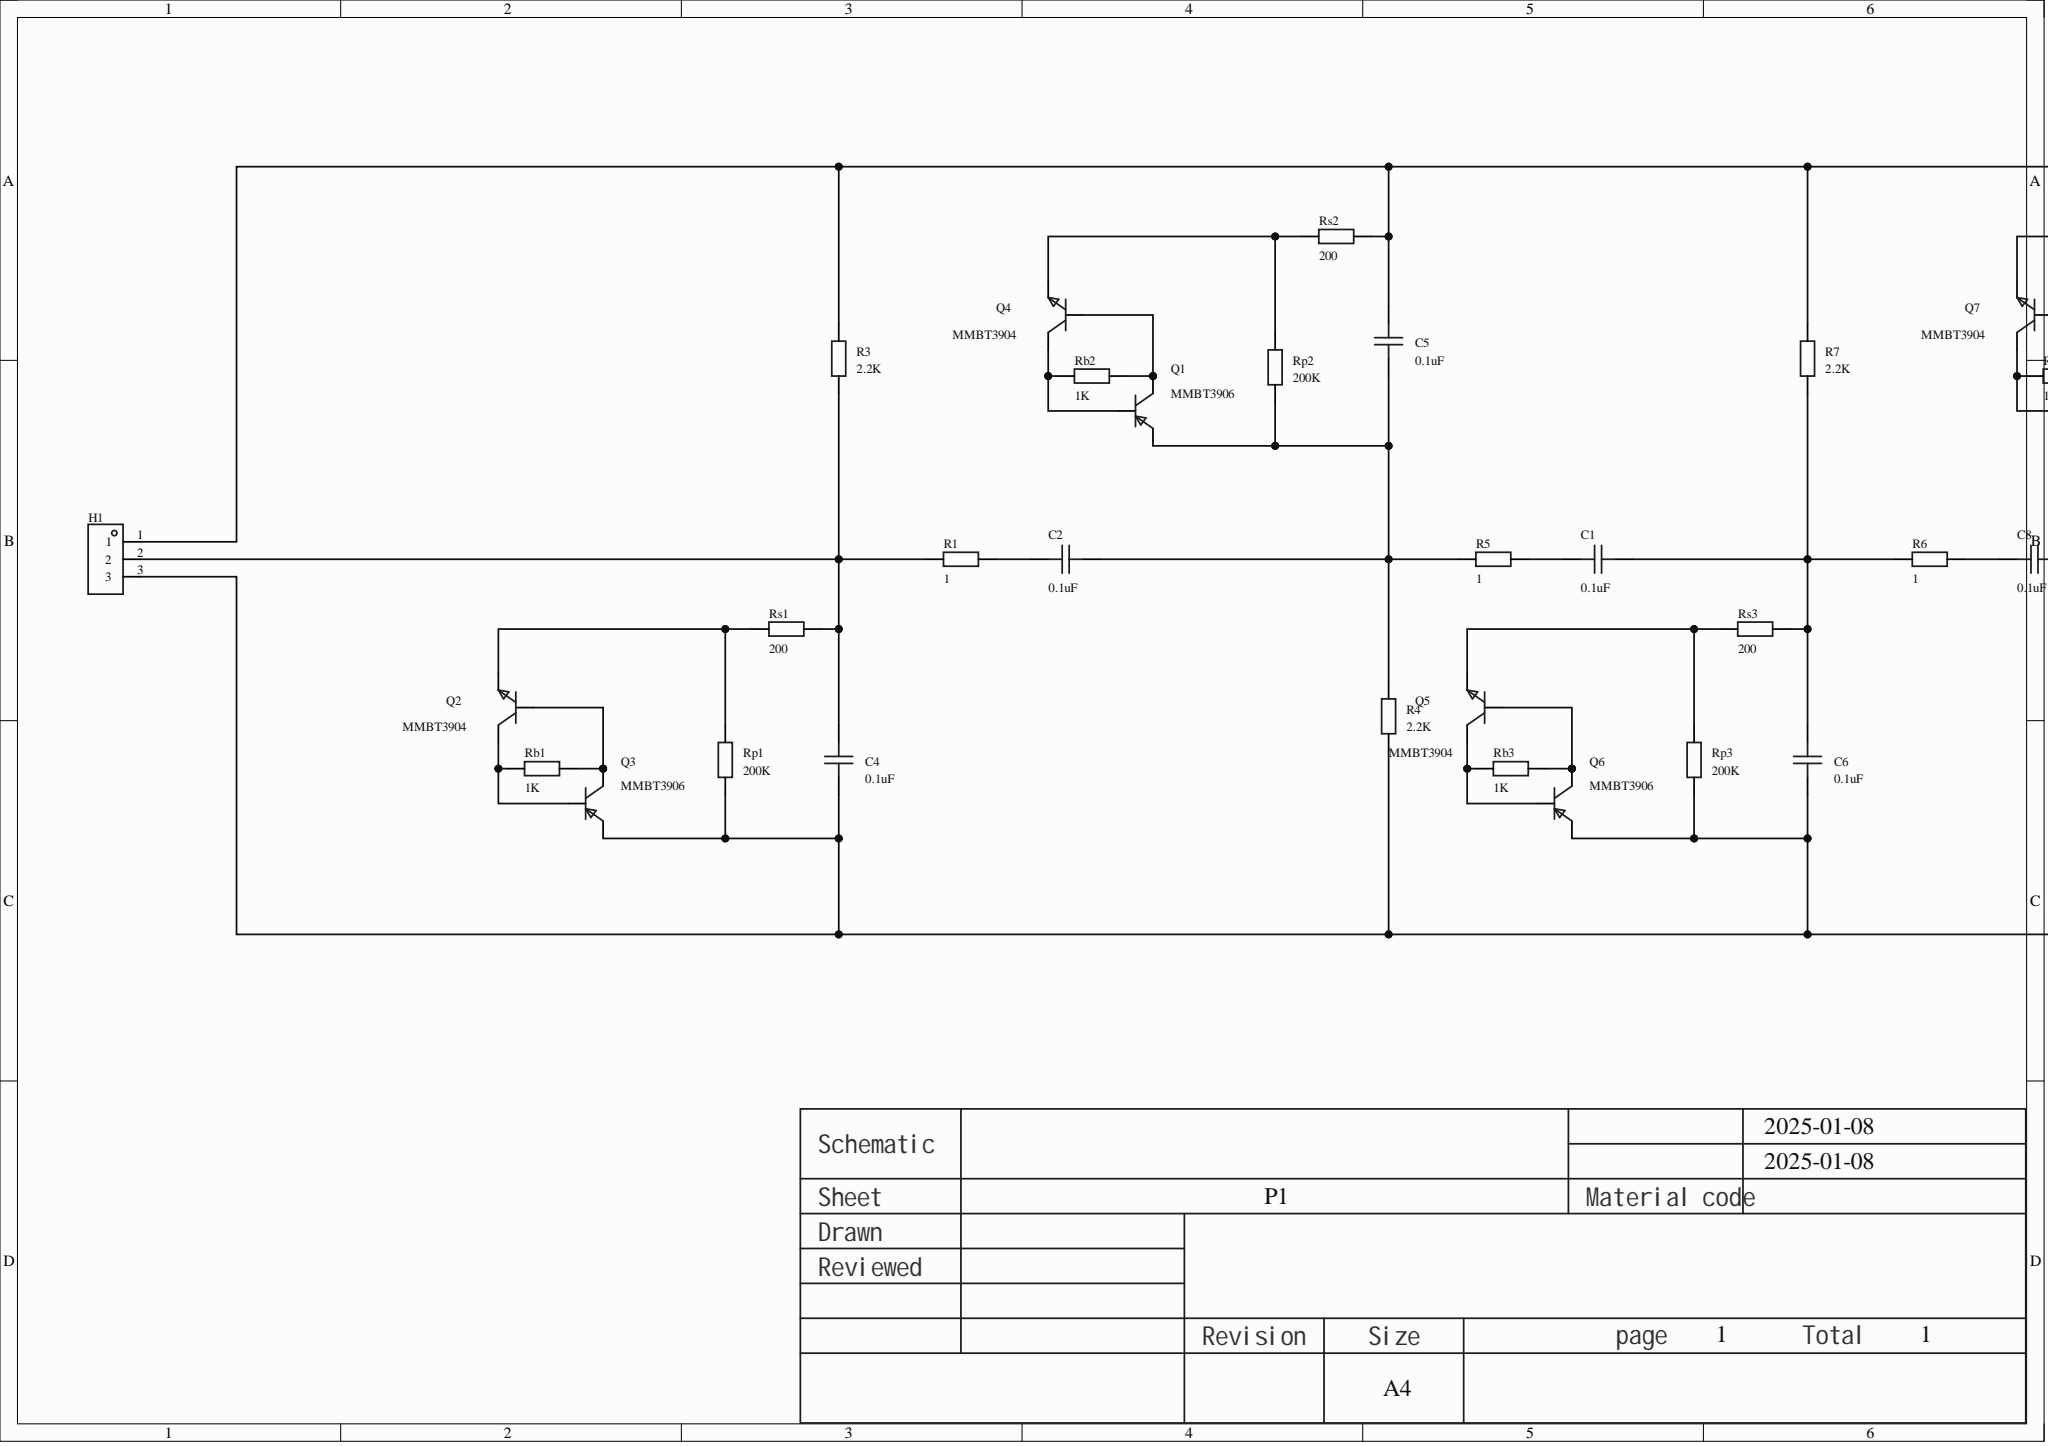Circuit board | Altium Designer | 257 parts | 141 nets
Bill of materials:
Comment,Description,Designator,Footprint,LibRef,Quantity
"0.1uF","","C1, C2, C4, C5, C6, C7, C8, C9, C10, C11, C12, C13, C14, C15, C16, C17, C18, C19, C20, C21, C22, C23, C24, C25, C26, C27, C28, C29, C30, C31, C32, C33, C34, C35, C36, C37, C38, C39, C40, C41, C42, C43, C44, C45, C46, C47, C48, C49, C50, C51, C52, C53, C54, C55, C56","C0402","CAP_0402","55"
"","","H1","HDR-TH_3P-P2.54-V-M","HDR-M_2.54_1x3P","1"
"","","H2, H3, H4, H5, H6, H7","HDR-TH_2P-P2.54-V-M-1","HDR-M_2.54_1x2P","6"
"MMBT3906","Transistor type:-;Collector current(Ic):-;Collector-emitter breakdown voltage(Vceo):-;Power(Pd):-;","Q1, Q3, Q6, Q8, Q10, Q12, Q14, Q16, Q18, Q20, Q22, Q24, Q26, Q28, Q30, Q32, Q34, Q36, Q38, Q40, Q42, Q44, Q46, Q48, Q50, Q52, Q54, Q56","SOT-23-3_L2.9-W1.3-P1.90-LS2.4-BR","MMBT3906-13-01-F","28"
"MMBT3904","晶体管类型:NPN;集电极电流(Ic):200mA;集射极击穿电压(Vceo):40V;功率(Pd):200mW;直流电流增益(hFE@Ic,Vce):100@10mA,1V;","Q2, Q4, Q5, Q7, Q9, Q11, Q13, Q15, Q17, Q19, Q21, Q23, Q25, Q27, Q29, Q31, Q33, Q35, Q37, Q39, Q41, Q43, Q45, Q47, Q49, Q51, Q53, Q55","SOT-23-3_L2.9-W1.3-P1.90-LS2.4-BR","MMBT3904(RANGE:100-300)","28"
"1","","R1, R5, R6, R8, R10, R12, R14, R16, R18, R20, R22, R24, R26, R28, R30, R32, R34, R36, R38, R40, R42, R44, R46, R48, R50, R52, R54","R0402","Res_0402","27"
"2.2K","","R3, R4, R7, R9, R11, R13, R15, R17, R19, R21, R23, R25, R27, R29, R31, R33, R35, R37, R39, R41, R43, R45, R47, R49, R51, R53, R55, R56","R0402","Res_0402","28"
"1K","","Rb1, Rb2, Rb3, Rb4, Rb5, Rb6, Rb7, Rb8, Rb9, Rb10, Rb11, Rb12, Rb13, Rb14, Rb15, Rb16, Rb17, Rb18, Rb19, Rb20, Rb21, Rb22, Rb23, Rb24, Rb25, Rb26, Rb27, Rb28","R0402","Res_0402","28"
"200K","","Rp1, Rp2, Rp3, Rp4, Rp5, Rp6, Rp7, Rp8, Rp9, Rp10, Rp11, Rp12, Rp13, Rp14, Rp15, Rp16, Rp17, Rp18, Rp19, Rp20, Rp21, Rp22, Rp23, Rp24, Rp25, Rp26, Rp27, Rp28","R0402","Res_0402","28"
"200","","Rs1, Rs2, Rs3, Rs4, Rs5, Rs6, Rs7, Rs8, Rs9, Rs10, Rs11, Rs12, Rs13, Rs14, Rs15, Rs16, Rs17, Rs18, Rs19, Rs20, Rs21, Rs22, Rs23, Rs24, Rs25, Rs26, Rs27, Rs28","R0402","Res_0402","28"
Netlist (Protel format):
[
C1
C0402
0.1uF



]
[
C2
C0402
0.1uF



]
[
C4
C0402
0.1uF



]
[
C5
C0402
0.1uF



]
[
C6
C0402
0.1uF



]
[
C7
C0402
0.1uF



]
[
C8
C0402
0.1uF



]
[
C9
C0402
0.1uF



]
[
C10
C0402
0.1uF



]
[
C11
C0402
0.1uF



]
[
C12
C0402
0.1uF



]
[
C13
C0402
0.1uF



]
[
C14
C0402
0.1uF



]
[
C15
C0402
0.1uF



]
[
C16
C0402
0.1uF



]
[
C17
C0402
0.1uF



]
[
C18
C0402
0.1uF



]
[
C19
C0402
0.1uF



]
[
C20
C0402
0.1uF



]
[
C21
C0402
0.1uF



]
[
C22
C0402
0.1uF



]
[
C23
C0402
0.1uF



]
[
C24
C0402
0.1uF



]
[
C25
C0402
0.1uF



]
[
C26
C0402
0.1uF



]
[
C27
C0402
0.1uF



]
[
C28
C0402
0.1uF



]
[
C29
C0402
0.1uF



]
[
C30
C0402
0.1uF



]
[
C31
C0402
0.1uF



]
[
C32
C0402
0.1uF



]
[
C33
C0402
0.1uF



]
[
C34
C0402
0.1uF



]
[
C35
C0402
0.1uF



]
[
C36
C0402
0.1uF



]
[
C37
C0402
0.1uF



]
[
C38
C0402
0.1uF



]
[
C39
C0402
0.1uF



]
[
C40
C0402
0.1uF



]
[
C41
C0402
0.1uF



]
[
C42
C0402
0.1uF



]
[
C43
C0402
0.1uF



]
[
C44
C0402
0.1uF



]
[
C45
C0402
0.1uF



]
[
C46
C0402
0.1uF



]
[
C47
C0402
0.1uF



]
[
C48
C0402
0.1uF



]
[
C49
C0402
0.1uF



]
[
C50
C0402
0.1uF



]
[
C51
C0402
0.1uF



]
[
C52
C0402
0.1uF



]
[
C53
C0402
0.1uF



]
[
C54
C0402
0.1uF



]
[
C55
C0402
0.1uF



]
[
C56
C0402
0.1uF



]
[
H1
HDR-TH_3P-P2.54-V-M




]
[
H2
HDR-TH_2P-P2.54-V-M-1




]
[
H3
HDR-TH_2P-P2.54-V-M-1




]
[
H4
HDR-TH_2P-P2.54-V-M-1




]
[
H5
HDR-TH_2P-P2.54-V-M-1




]
[
H6
HDR-TH_2P-P2.54-V-M-1




]
[
H7
HDR-TH_2P-P2.54-V-M-1




]
[
Q1
SOT-23-3_L2.9-W1.3-P1.90-LS2.4-BR
MMBT3906



]
[
Q2
SOT-23-3_L2.9-W1.3-P1.90-LS2.4-BR
MMBT3904



]
[
Q3
SOT-23-3_L2.9-W1.3-P1.90-LS2.4-BR
MMBT3906



]
[
Q4
SOT-23-3_L2.9-W1.3-P1.90-LS2.4-BR
MMBT3904



]
[
Q5
SOT-23-3_L2.9-W1.3-P1.90-LS2.4-BR
MMBT3904



]
[
Q6
SOT-23-3_L2.9-W1.3-P1.90-LS2.4-BR
MMBT3906



]
[
Q7
SOT-23-3_L2.9-W1.3-P1.90-LS2.4-BR
MMBT3904



]
[
Q8
SOT-23-3_L2.9-W1.3-P1.90-LS2.4-BR
MMBT3906



]
[
Q9
SOT-23-3_L2.9-W1.3-P1.90-LS2.4-BR
MMBT3904



]
[
Q10
SOT-23-3_L2.9-W1.3-P1.90-LS2.4-BR
MMBT3906



]
[
Q11
SOT-23-3_L2.9-W1.3-P1.90-LS2.4-BR
MMBT3904



]
[
Q12
SOT-23-3_L2.9-W1.3-P1.90-LS2.4-BR
MMBT3906



]
[
Q13
SOT-23-3_L2.9-W1.3-P1.90-LS2.4-BR
MMBT3904



]
[
Q14
SOT-23-3_L2.9-W1.3-P1.90-LS2.4-BR
MMBT3906



]
[
Q15
SOT-23-3_L2.9-W1.3-P1.90-LS2.4-BR
MMBT3904



]
[
Q16
SOT-23-3_L2.9-W1.3-P1.90-LS2.4-BR
MMBT3906



]
[
Q17
SOT-23-3_L2.9-W1.3-P1.90-LS2.4-BR
MMBT3904



]
[
Q18
SOT-23-3_L2.9-W1.3-P1.90-LS2.4-BR
MMBT3906



]
[
Q19
SOT-23-3_L2.9-W1.3-P1.90-LS2.4-BR
MMBT3904



]
[
Q20
SOT-23-3_L2.9-W1.3-P1.90-LS2.4-BR
MMBT3906



]
[
Q21
SOT-23-3_L2.9-W1.3-P1.90-LS2.4-BR
MMBT3904



]
[
Q22
SOT-23-3_L2.9-W1.3-P1.90-LS2.4-BR
MMBT3906



]
[
Q23
SOT-23-3_L2.9-W1.3-P1.90-LS2.4-BR
MMBT3904



]
[
Q24
SOT-23-3_L2.9-W1.3-P1.90-LS2.4-BR
MMBT3906



]
[
Q25
SOT-23-3_L2.9-W1.3-P1.90-LS2.4-BR
MMBT3904



]
[
Q26
SOT-23-3_L2.9-W1.3-P1.90-LS2.4-BR
MMBT3906



]
[
Q27
SOT-23-3_L2.9-W1.3-P1.90-LS2.4-BR
MMBT3904



]
[
Q28
SOT-23-3_L2.9-W1.3-P1.90-LS2.4-BR
MMBT3906



]
[
Q29
SOT-23-3_L2.9-W1.3-P1.90-LS2.4-BR
MMBT3904



]
[
Q30
SOT-23-3_L2.9-W1.3-P1.90-LS2.4-BR
MMBT3906



]
[
Q31
SOT-23-3_L2.9-W1.3-P1.90-LS2.4-BR
MMBT3904



]
[
Q32
SOT-23-3_L2.9-W1.3-P1.90-LS2.4-BR
MMBT3906



]
[
Q33
SOT-23-3_L2.9-W1.3-P1.90-LS2.4-BR
MMBT3904



]
[
Q34
SOT-23-3_L2.9-W1.3-P1.90-LS2.4-BR
MMBT3906



]
[
Q35
SOT-23-3_L2.9-W1.3-P1.90-LS2.4-BR
MMBT3904



]
[
Q36
SOT-23-3_L2.9-W1.3-P1.90-LS2.4-BR
MMBT3906



]
[
Q37
SOT-23-3_L2.9-W1.3-P1.90-LS2.4-BR
MMBT3904



]
[
Q38
SOT-23-3_L2.9-W1.3-P1.90-LS2.4-BR
MMBT3906



]
[
Q39
SOT-23-3_L2.9-W1.3-P1.90-LS2.4-BR
MMBT3904



]
[
Q40
SOT-23-3_L2.9-W1.3-P1.90-LS2.4-BR
MMBT3906



]
[
Q41
SOT-23-3_L2.9-W1.3-P1.90-LS2.4-BR
MMBT3904



]
[
Q42
SOT-23-3_L2.9-W1.3-P1.90-LS2.4-BR
MMBT3906



]
[
Q43
SOT-23-3_L2.9-W1.3-P1.90-LS2.4-BR
MMBT3904



]
[
Q44
SOT-23-3_L2.9-W1.3-P1.90-LS2.4-BR
MMBT3906



]
[
Q45
SOT-23-3_L2.9-W1.3-P1.90-LS2.4-BR
MMBT3904



]
[
Q46
SOT-23-3_L2.9-W1.3-P1.90-LS2.4-BR
MMBT3906



]
[
Q47
SOT-23-3_L2.9-W1.3-P1.90-LS2.4-BR
MMBT3904



]
[
Q48
SOT-23-3_L2.9-W1.3-P1.90-LS2.4-BR
MMBT3906



]
[
Q49
SOT-23-3_L2.9-W1.3-P1.90-LS2.4-BR
MMBT3904



]
[
Q50
SOT-23-3_L2.9-W1.3-P1.90-LS2.4-BR
MMBT3906



]
[
Q51
SOT-23-3_L2.9-W1.3-P1.90-LS2.4-BR
MMBT3904



]
[
Q52
SOT-23-3_L2.9-W1.3-P1.90-LS2.4-BR
MMBT3906



]
[
Q53
SOT-23-3_L2.9-W1.3-P1.90-LS2.4-BR
MMBT3904



]
[
Q54
SOT-23-3_L2.9-W1.3-P1.90-LS2.4-BR
MMBT3906



]
[
Q55
SOT-23-3_L2.9-W1.3-P1.90-LS2.4-BR
MMBT3904



]
[
Q56
SOT-23-3_L2.9-W1.3-P1.90-LS2.4-BR
MMBT3906



]
[
R1
R0402
1



]
[
R3
R0402
2.2K



]
[
R4
R0402
2.2K



]
[
R5
R0402
1



]
[
R6
R0402
1



]
[
R7
R0402
2.2K



]
[
R8
R0402
1



]
[
R9
R0402
2.2K



]
[
R10
R0402
1



]
[
R11
R0402
2.2K



]
[
R12
R0402
1



]
[
R13
R0402
2.2K



]
[
R14
R0402
1



]
[
R15
R0402
2.2K



]
[
R16
R0402
1



]
[
R17
R0402
2.2K



]
[
R18
R0402
1



]
[
R19
R0402
2.2K



]
[
R20
R0402
1



]
[
R21
R0402
2.2K



]
[
R22
R0402
1



]
[
R23
R0402
2.2K



]
[
R24
R0402
1



]
[
R25
R0402
2.2K



]
[
R26
R0402
1



]
[
R27
R0402
2.2K



]
[
R28
R0402
1



]
[
R29
R0402
2.2K



]
[
R30
R0402
1



]
[
R31
R0402
2.2K



]
[
R32
R0402
1



]
[
R33
R0402
2.2K



]
[
R34
R0402
1



]
[
R35
R0402
2.2K



]
[
R36
R0402
1



]
[
R37
R0402
2.2K



]
[
R38
R0402
1



]
[
R39
R0402
2.2K



]
[
R40
R0402
1



]
[
R41
R0402
2.2K



]
[
R42
R0402
1



]
[
R43
R0402
2.2K



]
[
R44
R0402
1



]
[
R45
R0402
2.2K



]
[
R46
R0402
1



]
[
R47
R0402
2.2K



]
[
R48
R0402
1



]
[
R49
R0402
2.2K



]
[
R50
R0402
1



]
[
R51
R0402
2.2K



]
[
R52
R0402
1



]
[
R53
R0402
2.2K



]
[
R54
R0402
1



]
[
R55
R0402
2.2K



]
[
R56
R0402
2.2K



]
[
Rb1
R0402
1K



]
[
Rb2
R0402
1K



]
[
Rb3
R0402
1K



]
[
Rb4
R0402
1K



]
[
Rb5
R0402
1K



]
[
Rb6
R0402
1K



]
[
Rb7
R0402
1K



]
[
Rb8
R0402
1K



]
[
Rb9
R0402
1K



]
[
Rb10
R0402
1K



]
[
Rb11
R0402
1K



]
[
Rb12
R0402
1K



]
[
Rb13
R0402
1K



]
[
Rb14
R0402
1K



]
[
Rb15
R0402
1K



]
[
Rb16
R0402
1K



]
[
Rb17
R0402
1K



]
[
Rb18
R0402
1K



]
[
Rb19
R0402
1K



]
[
Rb20
R0402
1K



]
[
Rb21
R0402
1K



]
[
Rb22
R0402
1K



]
[
Rb23
R0402
1K



]
[
Rb24
R0402
1K



]
[
Rb25
R0402
1K



]
[
Rb26
R0402
1K



]
[
Rb27
R0402
1K



]
[
Rb28
R0402
1K



]
[
Rp1
R0402
200K



]
[
Rp2
R0402
200K



]
[
Rp3
R0402
200K



]
[
Rp4
R0402
200K



]
[
Rp5
R0402
200K



]
[
Rp6
R0402
200K



]
[
Rp7
R0402
200K



]
[
Rp8
R0402
200K



]
[
Rp9
R0402
200K



]
[
Rp10
R0402
200K



]
[
Rp11
R0402
200K



]
[
Rp12
R0402
200K



]
[
Rp13
R0402
200K



]
[
Rp14
R0402
200K



]
[
Rp15
R0402
200K



]
[
Rp16
R0402
200K



]
[
Rp17
R0402
200K



]
[
Rp18
R0402
200K



]
[
Rp19
R0402
200K



]
[
Rp20
R0402
200K



]
[
Rp21
R0402
200K



]
[
Rp22
R0402
200K



]
[
Rp23
R0402
200K



]
[
Rp24
R0402
200K



]
[
Rp25
R0402
200K



]
[
Rp26
R0402
200K



]
[
Rp27
R0402
200K



]
[
Rp28
R0402
200K



]
[
Rs1
R0402
200



]
[
Rs2
R0402
200



]
[
Rs3
R0402
200



]
[
Rs4
R0402
200



]
[
Rs5
R0402
200



]
[
Rs6
R0402
200



]
[
Rs7
R0402
200



]
[
Rs8
R0402
200



]
[
Rs9
R0402
200



]
[
Rs10
R0402
200



]
[
Rs11
R0402
200



]
[
Rs12
R0402
200



]
[
Rs13
R0402
200



]
[
Rs14
R0402
200



]
[
Rs15
R0402
200



]
[
Rs16
R0402
200



]
[
Rs17
R0402
200



]
[
Rs18
R0402
200



]
[
Rs19
R0402
200



]
[
Rs20
R0402
200



]
[
Rs21
R0402
200



]
[
Rs22
R0402
200



]
[
Rs23
R0402
200



]
[
Rs24
R0402
200



]
[
Rs25
R0402
200



]
[
Rs26
R0402
200



]
[
Rs27
R0402
200



]
[
Rs28
R0402
200



]
(
NetQ55_3
Q55-3
Q56-1
Rb28-2
)
(
NetQ55_2
Q55-2
Rp28-2
Rs28-1
)
(
NetQ55_1
Q55-1
Q56-3
Rb28-1
)
(
NetQ53_3
Q53-3
Q54-1
Rb27-2
)
(
NetQ53_2
Q53-2
Rp27-2
Rs27-1
)
(
NetQ53_1
Q53-1
Q54-3
Rb27-1
)
(
NetQ51_3
Q51-3
Q52-1
Rb26-2
)
(
NetQ51_2
Q51-2
Rp26-2
Rs26-1
)
(
NetQ51_1
Q51-1
Q52-3
Rb26-1
)
(
NetQ49_3
Q49-3
Q50-1
Rb25-2
)
(
NetQ49_2
Q49-2
Rp25-2
Rs25-1
)
(
NetQ49_1
Q49-1
Q50-3
Rb25-1
)
(
NetQ47_3
Q47-3
Q48-1
Rb24-2
)
(
NetQ47_1
Q47-1
Q48-3
Rb24-1
)
(
NetQ45_3
Q45-3
Q46-1
Rb23-2
)
(
NetQ45_2
Q45-2
Rp23-2
Rs23-1
)
(
NetQ45_1
Q45-1
Q46-3
Rb23-1
)
(
NetQ43_3
Q43-3
Q44-1
Rb22-2
)
(
NetQ43_2
Q43-2
Rp22-2
Rs22-1
)
(
NetQ43_1
Q43-1
Q44-3
Rb22-1
)
(
NetQ41_3
Q41-3
Q42-1
Rb21-2
)
(
NetQ41_2
Q41-2
Rp21-2
Rs21-1
)
(
NetQ41_1
Q41-1
Q42-3
Rb21-1
)
(
NetQ39_3
Q39-3
Q40-1
Rb20-2
)
(
NetQ39_1
Q39-1
Q40-3
Rb20-1
)
(
NetQ37_3
Q37-3
Q38-1
Rb19-2
)
(
NetQ37_2
Q37-2
Rp19-2
Rs19-1
)
(
NetQ37_1
Q37-1
Q38-3
Rb19-1
)
(
NetQ35_3
Q35-3
Q36-1
Rb18-2
)
(
NetQ35_2
Q35-2
Rp18-2
Rs18-1
)
(
NetQ35_1
Q35-1
Q36-3
Rb18-1
)
(
NetQ33_3
Q33-3
Q34-1
Rb17-2
)
(
NetQ33_2
Q33-2
Rp17-2
Rs17-1
)
(
NetQ33_1
Q33-1
Q34-3
Rb17-1
)
(
NetQ31_3
Q31-3
Q32-1
Rb16-2
)
(
NetQ31_1
Q31-1
Q32-3
Rb16-1
)
(
NetQ29_3
Q29-3
Q30-1
Rb15-2
)
(
NetQ29_2
Q29-2
Rp15-2
Rs15-1
)
(
NetQ29_1
Q29-1
Q30-3
Rb15-1
)
(
NetQ27_3
Q27-3
Q28-1
Rb14-2
)
(
NetQ27_2
Q27-2
Rp14-2
Rs14-1
)
(
NetQ27_1
Q27-1
Q28-3
Rb14-1
)
(
NetQ25_3
Q25-3
Q26-1
Rb13-2
)
(
NetQ25_2
Q25-2
Rp13-2
Rs13-1
)
(
NetQ25_1
Q25-1
Q26-3
Rb13-1
)
(
NetQ23_3
Q23-3
Q24-1
Rb12-2
)
(
NetQ23_1
Q23-1
Q24-3
Rb12-1
)
(
NetQ21_3
Q21-3
Q22-1
Rb11-2
)
(
NetQ21_2
Q21-2
Rp11-2
Rs11-1
)
(
NetQ21_1
Q21-1
Q22-3
Rb11-1
)
(
NetQ19_3
Q19-3
Q20-1
Rb10-2
)
(
NetQ19_2
Q19-2
Rp10-2
Rs10-1
)
(
NetQ19_1
Q19-1
Q20-3
Rb10-1
)
(
NetQ17_3
Q17-3
Q18-1
Rb9-2
)
(
NetQ17_2
Q17-2
Rp9-2
Rs9-1
)
(
NetQ17_1
Q17-1
Q18-3
Rb9-1
)
(
NetQ15_3
Q15-3
Q16-1
Rb8-2
)
(
NetQ15_1
Q15-1
Q16-3
Rb8-1
)
(
NetQ13_3
Q13-3
Q14-1
Rb7-2
)
(
NetQ13_2
Q13-2
Rp7-2
Rs7-1
)
(
NetQ13_1
Q13-1
Q14-3
Rb7-1
)
(
NetQ11_3
Q11-3
Q12-1
Rb6-2
)
(
NetQ11_2
Q11-2
Rp6-2
Rs6-1
)
(
NetQ11_1
Q11-1
Q12-3
Rb6-1
)
(
NetQ9_3
Q9-3
Q10-1
Rb5-2
)
(
NetQ9_2
Q9-2
Rp5-2
Rs5-1
)
(
NetQ9_1
Q9-1
Q10-3
Rb5-1
)
(
NetQ7_3
Q7-3
Q8-1
Rb4-2
)
(
NetQ7_1
Q7-1
Q8-3
Rb4-1
)
(
NetQ5_3
Q5-3
Q6-1
Rb3-2
)
(
NetQ5_2
Q5-2
Rp3-2
Rs3-1
)
(
NetQ5_1
Q5-1
Q6-3
Rb3-1
)
(
NetQ4_2
Q4-2
Rp2-2
Rs2-1
)
(
NetQ2_3
Q2-3
Q3-1
Rb1-2
)
(
NetQ2_2
Q2-2
Rp1-2
Rs1-1
)
(
NetQ2_1
Q2-1
Q3-3
Rb1-1
)
(
NetQ1_3
Q1-3
Q4-1
Rb2-1
)
(
NetQ1_1
Q1-1
Q4-3
Rb2-2
)
(
NetH7_1
H7-1
Q47-2
Rp24-2
Rs24-1
)
(
NetH6_1
H6-1
Q39-2
Rp20-2
Rs20-1
)
(
NetH5_1
H5-1
Q31-2
Rp16-2
Rs16-1
)
(
NetH4_1
H4-1
Q23-2
Rp12-2
Rs12-1
)
(
NetH3_1
H3-1
Q15-2
Rp8-2
Rs8-1
)
(
NetH2_1
H2-1
Q7-2
Rp4-2
Rs4-1
)
(
NetC56_2
C56-2
R54-1
)
(
NetC55_1
C55-1
C56-1
Q56-2
R56-2
Rp28-1
)
(
NetC53_2
C53-2
R52-1
)
(
NetC53_1
C53-1
C54-2
R54-2
R55-1
Rs27-2
)
(
NetC52_2
C52-2
R50-1
)
(
NetC51_1
C51-1
C52-1
Q52-2
R52-2
R53-2
Rp26-1
)
(
NetC49_2
C49-2
R48-1
)
(
NetC49_1
C49-1
C50-2
H7-2
R50-2
R51-1
Rs25-2
)
(
NetC48_2
C48-2
R46-1
)
(
NetC47_1
C47-1
C48-1
Q48-2
R48-2
R49-2
Rp24-1
)
(
NetC45_2
C45-2
R44-1
)
(
NetC45_1
C45-1
C46-2
R46-2
R47-1
Rs23-2
)
(
NetC44_2
C44-2
R42-1
)
(
NetC43_1
C43-1
C44-1
Q44-2
R44-2
R45-2
Rp22-1
)
(
NetC41_2
C41-2
R40-1
)
(
NetC41_1
C41-1
C42-2
H6-2
R42-2
R43-1
Rs21-2
)
(
NetC40_2
C40-2
R38-1
)
(
NetC39_1
C39-1
C40-1
Q40-2
R40-2
R41-2
Rp20-1
)
(
NetC37_2
C37-2
R36-1
)
(
NetC37_1
C37-1
C38-2
R38-2
R39-1
Rs19-2
)
(
NetC36_2
C36-2
R34-1
)
(
NetC35_1
C35-1
C36-1
Q36-2
R36-2
R37-2
Rp18-1
)
(
NetC33_2
C33-2
R32-1
)
(
NetC33_1
C33-1
C34-2
H5-2
R34-2
R35-1
Rs17-2
)
(
NetC32_2
C32-2
R30-1
)
(
NetC31_1
C31-1
C32-1
Q32-2
R32-2
R33-2
Rp16-1
)
(
NetC29_2
C29-2
R28-1
)
(
NetC29_1
C29-1
C30-2
R30-2
R31-1
Rs15-2
)
(
NetC28_2
C28-2
R26-1
)
(
NetC27_1
C27-1
C28-1
Q28-2
R28-2
R29-2
Rp14-1
)
(
NetC25_2
C25-2
R24-1
)
(
NetC25_1
C25-1
C26-2
H4-2
R26-2
R27-1
Rs13-2
)
(
NetC24_2
C24-2
R22-1
)
(
NetC23_1
C23-1
C24-1
Q24-2
R24-2
R25-2
Rp12-1
)
(
NetC21_2
C21-2
R20-1
)
(
NetC21_1
C21-1
C22-2
R22-2
R23-1
Rs11-2
)
(
NetC20_2
C20-2
R18-1
)
(
NetC19_1
C19-1
C20-1
Q20-2
R20-2
R21-2
Rp10-1
)
(
NetC17_2
C17-2
R16-1
)
(
NetC17_1
C17-1
C18-2
H3-2
R18-2
R19-1
Rs9-2
)
(
NetC16_2
C16-2
R14-1
)
(
NetC15_1
C15-1
C16-1
Q16-2
R16-2
R17-2
Rp8-1
)
(
NetC13_2
C13-2
R12-1
)
(
NetC13_1
C13-1
C14-2
R14-2
R15-1
Rs7-2
)
(
NetC12_2
C12-2
R10-1
)
(
NetC11_1
C11-1
C12-1
Q12-2
R12-2
R13-2
Rp6-1
)
(
NetC9_2
C9-2
R8-1
)
(
NetC9_1
C9-1
C10-2
H2-2
R10-2
R11-1
Rs5-2
)
(
NetC8_2
C8-2
R6-1
)
(
NetC7_1
C7-1
C8-1
Q8-2
R8-2
R9-2
Rp4-1
)
(
NetC5_2
C5-2
C7-2
C11-2
C15-2
C19-2
C23-2
C27-2
C31-2
C35-2
C39-2
C43-2
C47-2
C51-2
C55-2
H1-1
R3-2
R7-2
R11-2
R15-2
R19-2
R23-2
R27-2
R31-2
R35-2
R39-2
R43-2
R47-2
R51-2
R55-2
Rs2-2
Rs4-2
Rs6-2
Rs8-2
Rs10-2
Rs12-2
Rs14-2
Rs16-2
Rs18-2
Rs20-2
Rs22-2
Rs24-2
Rs26-2
Rs28-2
)
(
NetC4_2
C4-2
H1-2
R1-2
R3-1
Rs1-2
)
(
NetC4_1
C4-1
C6-1
C10-1
C14-1
C18-1
C22-1
C26-1
C30-1
C34-1
C38-1
C42-1
C46-1
C50-1
C54-1
H1-3
Q3-2
Q6-2
Q10-2
Q14-2
Q18-2
Q22-2
Q26-2
Q30-2
Q34-2
Q38-2
Q42-2
Q46-2
Q50-2
Q54-2
R4-1
R9-1
R13-1
R17-1
R21-1
R25-1
R29-1
R33-1
R37-1
R41-1
R45-1
R49-1
R53-1
R56-1
Rp1-1
Rp3-1
Rp5-1
Rp7-1
Rp9-1
Rp11-1
Rp13-1
Rp15-1
Rp17-1
Rp19-1
Rp21-1
Rp23-1
Rp25-1
Rp27-1
)
(
NetC2_2
C2-2
R1-1
)
(
NetC2_1
C2-1
C5-1
Q1-2
R4-2
R5-2
Rp2-1
)
(
NetC1_2
C1-2
R5-1
)
(
NetC1_1
C1-1
C6-2
R6-2
R7-1
Rs3-2
)